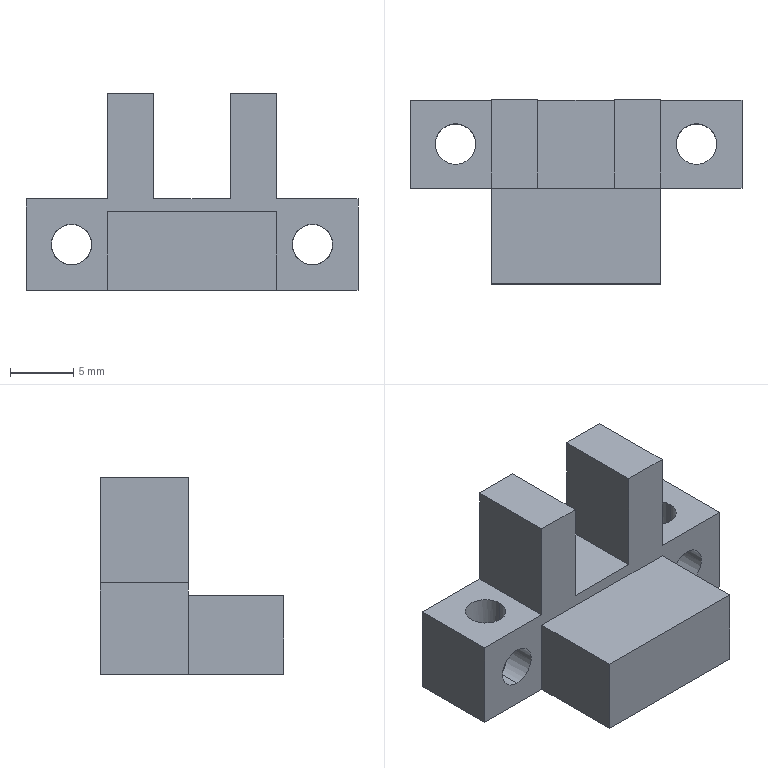Part | STEP file | 671 | 1 solid | 34 faces | box 26.18 x 14.5 x 15.5 mm | volume 2180 mm3 | plane 18 | cylinder 16 | commonest cylinder face diameters 3.2 x16